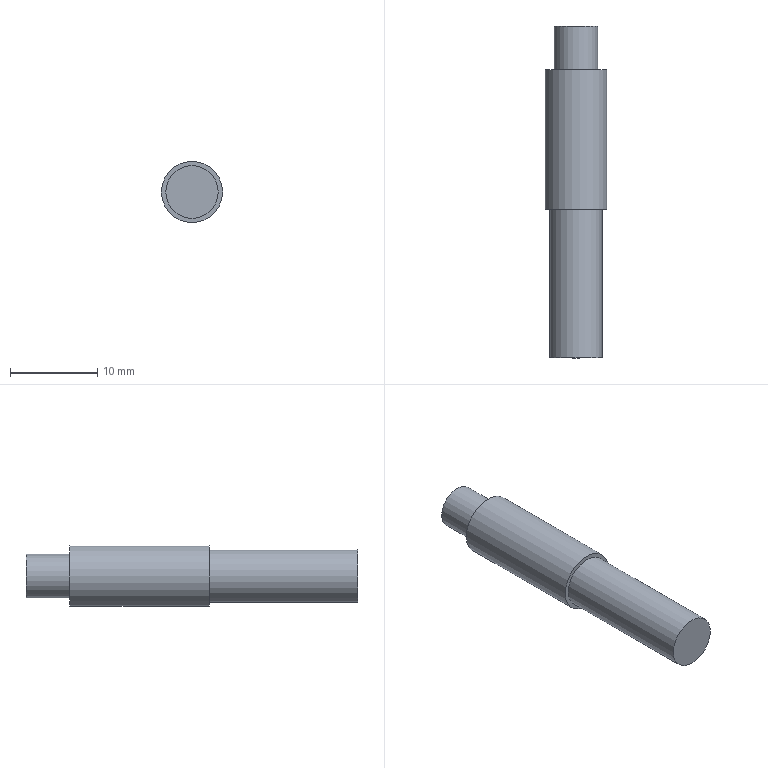Part | STEP file | 2-01.3 | 1 solid | 7 faces | box 7 x 38 x 7 mm | volume 1195 mm3 | plane 4 | cylinder 3 | commonest cylinder face diameters 5 x1 6 x1 7 x1
STEP:
#1=CARTESIAN_POINT('',(0.,0.,0.));
#2=DIRECTION('',(0.,0.,1.));
#3=DIRECTION('',(1.,0.,0.));
#4=AXIS2_PLACEMENT_3D('',#1,#2,#3);
#5=CARTESIAN_POINT('',(3.5,0.,0.));
#6=VERTEX_POINT('',#5);
#7=CARTESIAN_POINT('',(0.,0.,0.));
#8=DIRECTION('',(0.,-1.,0.));
#9=DIRECTION('',(1.,0.,0.));
#10=AXIS2_PLACEMENT_3D('',#7,#8,#9);
#11=CIRCLE('',#10,3.5);
#12=CARTESIAN_POINT('',(0.,0.,0.));
#13=DIRECTION('',(0.,-1.,0.));
#14=DIRECTION('',(1.,0.,0.));
#15=AXIS2_PLACEMENT_3D('',#12,#13,#14);
#16=CYLINDRICAL_SURFACE('',#15,3.5);
#17=CARTESIAN_POINT('',(0.,0.));
#18=DIRECTION('',(1.,0.));
#19=VECTOR('',#18,1.);
#20=LINE('',#17,#19);
#21=(GEOMETRIC_REPRESENTATION_CONTEXT(2)PARAMETRIC_REPRESENTATION_CONTEXT()REPRESENTATION_CONTEXT('',''));
#22=DEFINITIONAL_REPRESENTATION('',(#20),#21);
#23=PCURVE('',#16,#22);
#24=CARTESIAN_POINT('',(-0.9378,0.,0.));
#25=DIRECTION('',(0.,-1.,0.));
#26=DIRECTION('',(1.,0.,0.));
#27=AXIS2_PLACEMENT_3D('',#24,#25,#26);
#28=PLANE('',#27);
#29=CARTESIAN_POINT('',(0.9378,0.));
#30=DIRECTION('',(1.,0.));
#31=AXIS2_PLACEMENT_2D('',#29,#30);
#32=CIRCLE('',#31,3.5);
#33=(GEOMETRIC_REPRESENTATION_CONTEXT(2)PARAMETRIC_REPRESENTATION_CONTEXT()REPRESENTATION_CONTEXT('',''));
#34=DEFINITIONAL_REPRESENTATION('',(#32),#33);
#35=PCURVE('',#28,#34);
#36=SURFACE_CURVE('',#11,(#23,#35),.PCURVE_S1.);
#37=EDGE_CURVE('',#6,#6,#36,.T.);
#38=ORIENTED_EDGE('',*,*,#37,.T.);
#39=CARTESIAN_POINT('',(3.5,-16.,0.));
#40=VERTEX_POINT('',#39);
#41=CARTESIAN_POINT('',(3.5,0.,0.));
#42=DIRECTION('',(0.,-1.,0.));
#43=VECTOR('',#42,1.);
#44=LINE('',#41,#43);
#45=CARTESIAN_POINT('',(6.283,0.));
#46=DIRECTION('',(0.,1.));
#47=VECTOR('',#46,1.);
#48=LINE('',#45,#47);
#49=(GEOMETRIC_REPRESENTATION_CONTEXT(2)PARAMETRIC_REPRESENTATION_CONTEXT()REPRESENTATION_CONTEXT('',''));
#50=DEFINITIONAL_REPRESENTATION('',(#48),#49);
#51=PCURVE('',#16,#50);
#52=CARTESIAN_POINT('',(0.,0.));
#53=DIRECTION('',(0.,1.));
#54=VECTOR('',#53,1.);
#55=LINE('',#52,#54);
#56=(GEOMETRIC_REPRESENTATION_CONTEXT(2)PARAMETRIC_REPRESENTATION_CONTEXT()REPRESENTATION_CONTEXT('',''));
#57=DEFINITIONAL_REPRESENTATION('',(#55),#56);
#58=PCURVE('',#16,#57);
#59=SEAM_CURVE('',#44,(#51,#58),.PCURVE_S1.);
#60=EDGE_CURVE('',#6,#40,#59,.T.);
#61=ORIENTED_EDGE('',*,*,#60,.T.);
#62=CARTESIAN_POINT('',(0.,-16.,0.));
#63=DIRECTION('',(0.,-1.,0.));
#64=DIRECTION('',(1.,0.,0.));
#65=AXIS2_PLACEMENT_3D('',#62,#63,#64);
#66=CIRCLE('',#65,3.5);
#67=CARTESIAN_POINT('',(0.,16.));
#68=DIRECTION('',(1.,0.));
#69=VECTOR('',#68,1.);
#70=LINE('',#67,#69);
#71=(GEOMETRIC_REPRESENTATION_CONTEXT(2)PARAMETRIC_REPRESENTATION_CONTEXT()REPRESENTATION_CONTEXT('',''));
#72=DEFINITIONAL_REPRESENTATION('',(#70),#71);
#73=PCURVE('',#16,#72);
#74=CARTESIAN_POINT('',(-0.9378,-16.,0.));
#75=DIRECTION('',(0.,-1.,0.));
#76=DIRECTION('',(1.,0.,0.));
#77=AXIS2_PLACEMENT_3D('',#74,#75,#76);
#78=PLANE('',#77);
#79=CARTESIAN_POINT('',(0.9378,0.));
#80=DIRECTION('',(1.,0.));
#81=AXIS2_PLACEMENT_2D('',#79,#80);
#82=CIRCLE('',#81,3.5);
#83=(GEOMETRIC_REPRESENTATION_CONTEXT(2)PARAMETRIC_REPRESENTATION_CONTEXT()REPRESENTATION_CONTEXT('',''));
#84=DEFINITIONAL_REPRESENTATION('',(#82),#83);
#85=PCURVE('',#78,#84);
#86=SURFACE_CURVE('',#66,(#73,#85),.PCURVE_S1.);
#87=EDGE_CURVE('',#40,#40,#86,.T.);
#88=ORIENTED_EDGE('',*,*,#87,.F.);
#89=ORIENTED_EDGE('',*,*,#60,.F.);
#90=EDGE_LOOP('',(#38,#61,#88,#89));
#91=FACE_BOUND('',#90,.T.);
#92=ADVANCED_FACE('',(#91),#16,.T.);
#93=ORIENTED_EDGE('',*,*,#87,.T.);
#94=EDGE_LOOP('',(#93));
#95=FACE_BOUND('',#94,.T.);
#96=CARTESIAN_POINT('',(3.,-16.,0.));
#97=VERTEX_POINT('',#96);
#98=CARTESIAN_POINT('',(0.,-16.,0.));
#99=DIRECTION('',(0.,-1.,0.));
#100=DIRECTION('',(1.,0.,0.));
#101=AXIS2_PLACEMENT_3D('',#98,#99,#100);
#102=CIRCLE('',#101,3.);
#103=CARTESIAN_POINT('',(0.9378,0.));
#104=DIRECTION('',(1.,0.));
#105=AXIS2_PLACEMENT_2D('',#103,#104);
#106=CIRCLE('',#105,3.);
#107=(GEOMETRIC_REPRESENTATION_CONTEXT(2)PARAMETRIC_REPRESENTATION_CONTEXT()REPRESENTATION_CONTEXT('',''));
#108=DEFINITIONAL_REPRESENTATION('',(#106),#107);
#109=PCURVE('',#78,#108);
#110=CARTESIAN_POINT('',(0.,-16.,0.));
#111=DIRECTION('',(0.,-1.,0.));
#112=DIRECTION('',(1.,0.,0.));
#113=AXIS2_PLACEMENT_3D('',#110,#111,#112);
#114=CYLINDRICAL_SURFACE('',#113,3.);
#115=CARTESIAN_POINT('',(0.,0.));
#116=DIRECTION('',(1.,0.));
#117=VECTOR('',#116,1.);
#118=LINE('',#115,#117);
#119=(GEOMETRIC_REPRESENTATION_CONTEXT(2)PARAMETRIC_REPRESENTATION_CONTEXT()REPRESENTATION_CONTEXT('',''));
#120=DEFINITIONAL_REPRESENTATION('',(#118),#119);
#121=PCURVE('',#114,#120);
#122=SURFACE_CURVE('',#102,(#109,#121),.PCURVE_S1.);
#123=EDGE_CURVE('',#97,#97,#122,.T.);
#124=ORIENTED_EDGE('',*,*,#123,.F.);
#125=EDGE_LOOP('',(#124));
#126=FACE_BOUND('',#125,.T.);
#127=ADVANCED_FACE('',(#95,#126),#78,.T.);
#128=ORIENTED_EDGE('',*,*,#123,.T.);
#129=CARTESIAN_POINT('',(3.,-33.,0.));
#130=VERTEX_POINT('',#129);
#131=CARTESIAN_POINT('',(3.,-16.,0.));
#132=DIRECTION('',(0.,-1.,0.));
#133=VECTOR('',#132,1.);
#134=LINE('',#131,#133);
#135=CARTESIAN_POINT('',(6.283,0.));
#136=DIRECTION('',(0.,1.));
#137=VECTOR('',#136,1.);
#138=LINE('',#135,#137);
#139=(GEOMETRIC_REPRESENTATION_CONTEXT(2)PARAMETRIC_REPRESENTATION_CONTEXT()REPRESENTATION_CONTEXT('',''));
#140=DEFINITIONAL_REPRESENTATION('',(#138),#139);
#141=PCURVE('',#114,#140);
#142=CARTESIAN_POINT('',(0.,0.));
#143=DIRECTION('',(0.,1.));
#144=VECTOR('',#143,1.);
#145=LINE('',#142,#144);
#146=(GEOMETRIC_REPRESENTATION_CONTEXT(2)PARAMETRIC_REPRESENTATION_CONTEXT()REPRESENTATION_CONTEXT('',''));
#147=DEFINITIONAL_REPRESENTATION('',(#145),#146);
#148=PCURVE('',#114,#147);
#149=SEAM_CURVE('',#134,(#141,#148),.PCURVE_S1.);
#150=EDGE_CURVE('',#97,#130,#149,.T.);
#151=ORIENTED_EDGE('',*,*,#150,.T.);
#152=CARTESIAN_POINT('',(0.,-33.,0.));
#153=DIRECTION('',(0.,-1.,0.));
#154=DIRECTION('',(1.,0.,0.));
#155=AXIS2_PLACEMENT_3D('',#152,#153,#154);
#156=CIRCLE('',#155,3.);
#157=CARTESIAN_POINT('',(0.,17.));
#158=DIRECTION('',(1.,0.));
#159=VECTOR('',#158,1.);
#160=LINE('',#157,#159);
#161=(GEOMETRIC_REPRESENTATION_CONTEXT(2)PARAMETRIC_REPRESENTATION_CONTEXT()REPRESENTATION_CONTEXT('',''));
#162=DEFINITIONAL_REPRESENTATION('',(#160),#161);
#163=PCURVE('',#114,#162);
#164=CARTESIAN_POINT('',(-0.8038,-33.,0.));
#165=DIRECTION('',(0.,-1.,0.));
#166=DIRECTION('',(1.,0.,0.));
#167=AXIS2_PLACEMENT_3D('',#164,#165,#166);
#168=PLANE('',#167);
#169=CARTESIAN_POINT('',(0.8038,0.));
#170=DIRECTION('',(1.,0.));
#171=AXIS2_PLACEMENT_2D('',#169,#170);
#172=CIRCLE('',#171,3.);
#173=(GEOMETRIC_REPRESENTATION_CONTEXT(2)PARAMETRIC_REPRESENTATION_CONTEXT()REPRESENTATION_CONTEXT('',''));
#174=DEFINITIONAL_REPRESENTATION('',(#172),#173);
#175=PCURVE('',#168,#174);
#176=SURFACE_CURVE('',#156,(#163,#175),.PCURVE_S1.);
#177=EDGE_CURVE('',#130,#130,#176,.T.);
#178=ORIENTED_EDGE('',*,*,#177,.F.);
#179=ORIENTED_EDGE('',*,*,#150,.F.);
#180=EDGE_LOOP('',(#128,#151,#178,#179));
#181=FACE_BOUND('',#180,.T.);
#182=ADVANCED_FACE('',(#181),#114,.T.);
#183=ORIENTED_EDGE('',*,*,#177,.T.);
#184=EDGE_LOOP('',(#183));
#185=FACE_BOUND('',#184,.T.);
#186=ADVANCED_FACE('',(#185),#168,.T.);
#187=ORIENTED_EDGE('',*,*,#37,.T.);
#188=EDGE_LOOP('',(#187));
#189=FACE_BOUND('',#188,.F.);
#190=CARTESIAN_POINT('',(2.5,0.,0.));
#191=VERTEX_POINT('',#190);
#192=CARTESIAN_POINT('',(0.,0.,0.));
#193=DIRECTION('',(0.,-1.,0.));
#194=DIRECTION('',(1.,0.,0.));
#195=AXIS2_PLACEMENT_3D('',#192,#193,#194);
#196=CIRCLE('',#195,2.5);
#197=CARTESIAN_POINT('',(0.9378,0.));
#198=DIRECTION('',(1.,0.));
#199=AXIS2_PLACEMENT_2D('',#197,#198);
#200=CIRCLE('',#199,2.5);
#201=(GEOMETRIC_REPRESENTATION_CONTEXT(2)PARAMETRIC_REPRESENTATION_CONTEXT()REPRESENTATION_CONTEXT('',''));
#202=DEFINITIONAL_REPRESENTATION('',(#200),#201);
#203=PCURVE('',#28,#202);
#204=CARTESIAN_POINT('',(0.,0.,0.));
#205=DIRECTION('',(0.,1.,0.));
#206=DIRECTION('',(1.,0.,0.));
#207=AXIS2_PLACEMENT_3D('',#204,#205,#206);
#208=CYLINDRICAL_SURFACE('',#207,2.5);
#209=CARTESIAN_POINT('',(6.283,0.));
#210=DIRECTION('',(-1.,0.));
#211=VECTOR('',#210,1.);
#212=LINE('',#209,#211);
#213=(GEOMETRIC_REPRESENTATION_CONTEXT(2)PARAMETRIC_REPRESENTATION_CONTEXT()REPRESENTATION_CONTEXT('',''));
#214=DEFINITIONAL_REPRESENTATION('',(#212),#213);
#215=PCURVE('',#208,#214);
#216=SURFACE_CURVE('',#196,(#203,#215),.PCURVE_S1.);
#217=EDGE_CURVE('',#191,#191,#216,.T.);
#218=ORIENTED_EDGE('',*,*,#217,.F.);
#219=EDGE_LOOP('',(#218));
#220=FACE_BOUND('',#219,.F.);
#221=ADVANCED_FACE('',(#189,#220),#28,.F.);
#222=CARTESIAN_POINT('',(2.5,5.,0.));
#223=VERTEX_POINT('',#222);
#224=CARTESIAN_POINT('',(2.5,0.,0.));
#225=DIRECTION('',(0.,1.,0.));
#226=VECTOR('',#225,1.);
#227=LINE('',#224,#226);
#228=CARTESIAN_POINT('',(6.283,0.));
#229=DIRECTION('',(0.,1.));
#230=VECTOR('',#229,1.);
#231=LINE('',#228,#230);
#232=(GEOMETRIC_REPRESENTATION_CONTEXT(2)PARAMETRIC_REPRESENTATION_CONTEXT()REPRESENTATION_CONTEXT('',''));
#233=DEFINITIONAL_REPRESENTATION('',(#231),#232);
#234=PCURVE('',#208,#233);
#235=CARTESIAN_POINT('',(0.,0.));
#236=DIRECTION('',(0.,1.));
#237=VECTOR('',#236,1.);
#238=LINE('',#235,#237);
#239=(GEOMETRIC_REPRESENTATION_CONTEXT(2)PARAMETRIC_REPRESENTATION_CONTEXT()REPRESENTATION_CONTEXT('',''));
#240=DEFINITIONAL_REPRESENTATION('',(#238),#239);
#241=PCURVE('',#208,#240);
#242=SEAM_CURVE('',#227,(#234,#241),.PCURVE_S1.);
#243=EDGE_CURVE('',#191,#223,#242,.T.);
#244=ORIENTED_EDGE('',*,*,#243,.T.);
#245=CARTESIAN_POINT('',(0.,5.,0.));
#246=DIRECTION('',(0.,-1.,0.));
#247=DIRECTION('',(1.,0.,0.));
#248=AXIS2_PLACEMENT_3D('',#245,#246,#247);
#249=CIRCLE('',#248,2.5);
#250=CARTESIAN_POINT('',(6.283,5.));
#251=DIRECTION('',(-1.,0.));
#252=VECTOR('',#251,1.);
#253=LINE('',#250,#252);
#254=(GEOMETRIC_REPRESENTATION_CONTEXT(2)PARAMETRIC_REPRESENTATION_CONTEXT()REPRESENTATION_CONTEXT('',''));
#255=DEFINITIONAL_REPRESENTATION('',(#253),#254);
#256=PCURVE('',#208,#255);
#257=CARTESIAN_POINT('',(-0.6699,5.,0.));
#258=DIRECTION('',(0.,-1.,0.));
#259=DIRECTION('',(1.,0.,0.));
#260=AXIS2_PLACEMENT_3D('',#257,#258,#259);
#261=PLANE('',#260);
#262=CARTESIAN_POINT('',(0.6699,0.));
#263=DIRECTION('',(1.,0.));
#264=AXIS2_PLACEMENT_2D('',#262,#263);
#265=CIRCLE('',#264,2.5);
#266=(GEOMETRIC_REPRESENTATION_CONTEXT(2)PARAMETRIC_REPRESENTATION_CONTEXT()REPRESENTATION_CONTEXT('',''));
#267=DEFINITIONAL_REPRESENTATION('',(#265),#266);
#268=PCURVE('',#261,#267);
#269=SURFACE_CURVE('',#249,(#256,#268),.PCURVE_S1.);
#270=EDGE_CURVE('',#223,#223,#269,.T.);
#271=ORIENTED_EDGE('',*,*,#270,.T.);
#272=ORIENTED_EDGE('',*,*,#243,.F.);
#273=ORIENTED_EDGE('',*,*,#217,.F.);
#274=EDGE_LOOP('',(#244,#271,#272,#273));
#275=FACE_BOUND('',#274,.T.);
#276=ADVANCED_FACE('',(#275),#208,.T.);
#277=ORIENTED_EDGE('',*,*,#270,.T.);
#278=EDGE_LOOP('',(#277));
#279=FACE_BOUND('',#278,.F.);
#280=ADVANCED_FACE('',(#279),#261,.F.);
#281=CLOSED_SHELL('',(#92,#127,#182,#186,#221,#276,#280));
#282=MANIFOLD_SOLID_BREP('',#281);
#283=(LENGTH_UNIT()NAMED_UNIT(*)SI_UNIT(.MILLI.,.METRE.));
#284=UNCERTAINTY_MEASURE_WITH_UNIT(LENGTH_MEASURE(0.0000001),#283,'','');
#285=(NAMED_UNIT(*)PLANE_ANGLE_UNIT()SI_UNIT($,.RADIAN.));
#286=(NAMED_UNIT(*)SI_UNIT($,.STERADIAN.)SOLID_ANGLE_UNIT());
#287=(GEOMETRIC_REPRESENTATION_CONTEXT(3)GLOBAL_UNCERTAINTY_ASSIGNED_CONTEXT((#284))GLOBAL_UNIT_ASSIGNED_CONTEXT((#283,#285,#286))REPRESENTATION_CONTEXT('',''));
#288=ADVANCED_BREP_SHAPE_REPRESENTATION('',(#4,#282),#287);